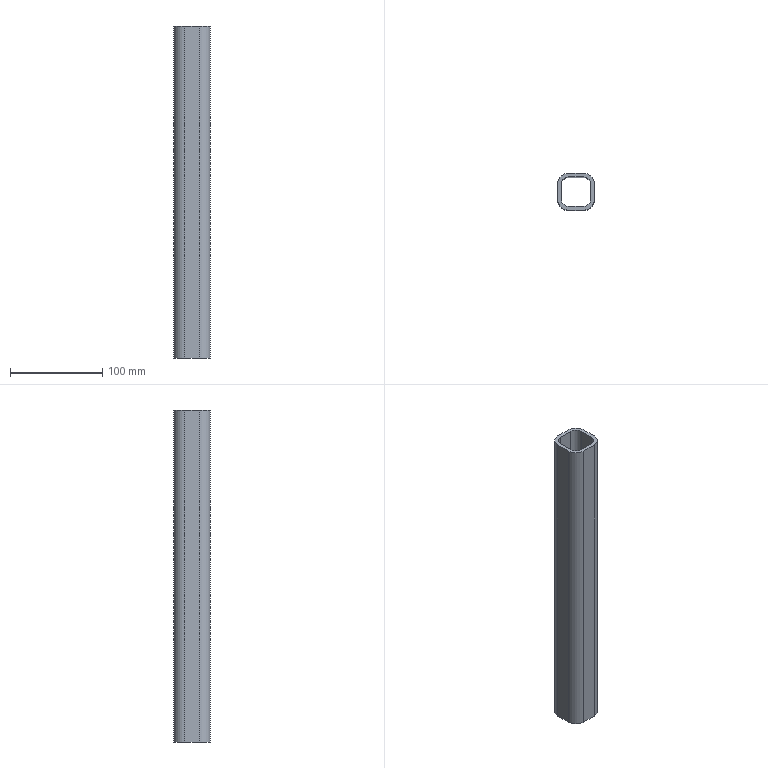Part | SolidWorks | features BaseBody 1 | 1 solid | 18 faces | box 40 x 40 x 360 mm | volume 182638 mm3 | plane 10 | cylinder 8 | commonest cylinder face diameters 16 x4 24 x4
STEP:
#1=CARTESIAN_POINT('',(8.,-20.,0.));
#2=VERTEX_POINT('',#1);
#3=CARTESIAN_POINT('',(20.,-8.,0.));
#4=VERTEX_POINT('',#3);
#5=CARTESIAN_POINT('',(8.,-8.,0.));
#6=DIRECTION('',(0.,0.,1.));
#7=DIRECTION('',(1.,0.,0.));
#8=AXIS2_PLACEMENT_3D('',#5,#6,#7);
#9=CIRCLE('',#8,12.);
#10=EDGE_CURVE('',#2,#4,#9,.T.);
#11=ORIENTED_EDGE('',*,*,#10,.T.);
#12=CARTESIAN_POINT('',(20.,-8.,360.));
#13=VERTEX_POINT('',#12);
#14=CARTESIAN_POINT('',(20.,-8.,0.));
#15=DIRECTION('',(0.,0.,1.));
#16=VECTOR('',#15,1000.);
#17=LINE('',#14,#16);
#18=EDGE_CURVE('',#4,#13,#17,.T.);
#19=ORIENTED_EDGE('',*,*,#18,.T.);
#20=CARTESIAN_POINT('',(8.,-20.,360.));
#21=VERTEX_POINT('',#20);
#22=CARTESIAN_POINT('',(8.,-8.,360.));
#23=DIRECTION('',(0.,0.,-1.));
#24=DIRECTION('',(1.,0.,0.));
#25=AXIS2_PLACEMENT_3D('',#22,#23,#24);
#26=CIRCLE('',#25,12.);
#27=EDGE_CURVE('',#13,#21,#26,.T.);
#28=ORIENTED_EDGE('',*,*,#27,.T.);
#29=CARTESIAN_POINT('',(8.,-20.,0.));
#30=DIRECTION('',(0.,0.,-1.));
#31=VECTOR('',#30,1000.);
#32=LINE('',#29,#31);
#33=EDGE_CURVE('',#21,#2,#32,.T.);
#34=ORIENTED_EDGE('',*,*,#33,.T.);
#35=EDGE_LOOP('',(#11,#19,#28,#34));
#36=FACE_OUTER_BOUND('',#35,.T.);
#37=CARTESIAN_POINT('',(8.,-8.,0.));
#38=DIRECTION('',(0.,0.,1.));
#39=DIRECTION('',(1.,0.,0.));
#40=AXIS2_PLACEMENT_3D('',#37,#38,#39);
#41=CYLINDRICAL_SURFACE('',#40,12.);
#42=ADVANCED_FACE('',(#36),#41,.T.);
#43=CARTESIAN_POINT('',(20.,8.,0.));
#44=VERTEX_POINT('',#43);
#45=CARTESIAN_POINT('',(20.,8.,0.));
#46=DIRECTION('',(0.,1.,0.));
#47=VECTOR('',#46,1000.);
#48=LINE('',#45,#47);
#49=EDGE_CURVE('',#4,#44,#48,.T.);
#50=ORIENTED_EDGE('',*,*,#49,.T.);
#51=CARTESIAN_POINT('',(20.,8.,360.));
#52=VERTEX_POINT('',#51);
#53=CARTESIAN_POINT('',(20.,8.,0.));
#54=DIRECTION('',(0.,0.,1.));
#55=VECTOR('',#54,1000.);
#56=LINE('',#53,#55);
#57=EDGE_CURVE('',#44,#52,#56,.T.);
#58=ORIENTED_EDGE('',*,*,#57,.T.);
#59=CARTESIAN_POINT('',(20.,8.,360.));
#60=DIRECTION('',(0.,-1.,0.));
#61=VECTOR('',#60,1000.);
#62=LINE('',#59,#61);
#63=EDGE_CURVE('',#52,#13,#62,.T.);
#64=ORIENTED_EDGE('',*,*,#63,.T.);
#65=ORIENTED_EDGE('',*,*,#18,.F.);
#66=EDGE_LOOP('',(#50,#58,#64,#65));
#67=FACE_OUTER_BOUND('',#66,.T.);
#68=CARTESIAN_POINT('',(20.,8.,0.));
#69=DIRECTION('',(1.,0.,0.));
#70=DIRECTION('',(0.,1.,0.));
#71=AXIS2_PLACEMENT_3D('',#68,#69,#70);
#72=PLANE('',#71);
#73=ADVANCED_FACE('',(#67),#72,.T.);
#74=CARTESIAN_POINT('',(-16.,8.,0.));
#75=VERTEX_POINT('',#74);
#76=CARTESIAN_POINT('',(-8.,16.,0.));
#77=VERTEX_POINT('',#76);
#78=CARTESIAN_POINT('',(-8.,8.,0.));
#79=DIRECTION('',(0.,0.,-1.));
#80=DIRECTION('',(1.,0.,0.));
#81=AXIS2_PLACEMENT_3D('',#78,#79,#80);
#82=CIRCLE('',#81,8.);
#83=EDGE_CURVE('',#75,#77,#82,.T.);
#84=ORIENTED_EDGE('',*,*,#83,.F.);
#85=CARTESIAN_POINT('',(-16.,-8.,0.));
#86=VERTEX_POINT('',#85);
#87=CARTESIAN_POINT('',(-16.,0.,0.));
#88=DIRECTION('',(0.,1.,0.));
#89=VECTOR('',#88,1000.);
#90=LINE('',#87,#89);
#91=EDGE_CURVE('',#86,#75,#90,.T.);
#92=ORIENTED_EDGE('',*,*,#91,.F.);
#93=CARTESIAN_POINT('',(-8.,-16.,0.));
#94=VERTEX_POINT('',#93);
#95=CARTESIAN_POINT('',(-8.,-8.,0.));
#96=DIRECTION('',(0.,0.,-1.));
#97=DIRECTION('',(1.,0.,0.));
#98=AXIS2_PLACEMENT_3D('',#95,#96,#97);
#99=CIRCLE('',#98,8.);
#100=EDGE_CURVE('',#94,#86,#99,.T.);
#101=ORIENTED_EDGE('',*,*,#100,.F.);
#102=CARTESIAN_POINT('',(8.,-16.,0.));
#103=VERTEX_POINT('',#102);
#104=CARTESIAN_POINT('',(0.,-16.,0.));
#105=DIRECTION('',(-1.,0.,0.));
#106=VECTOR('',#105,1000.);
#107=LINE('',#104,#106);
#108=EDGE_CURVE('',#103,#94,#107,.T.);
#109=ORIENTED_EDGE('',*,*,#108,.F.);
#110=CARTESIAN_POINT('',(16.,-8.,0.));
#111=VERTEX_POINT('',#110);
#112=CARTESIAN_POINT('',(8.,-8.,0.));
#113=DIRECTION('',(0.,0.,-1.));
#114=DIRECTION('',(1.,0.,0.));
#115=AXIS2_PLACEMENT_3D('',#112,#113,#114);
#116=CIRCLE('',#115,8.);
#117=EDGE_CURVE('',#111,#103,#116,.T.);
#118=ORIENTED_EDGE('',*,*,#117,.F.);
#119=CARTESIAN_POINT('',(16.,8.,0.));
#120=VERTEX_POINT('',#119);
#121=CARTESIAN_POINT('',(16.,0.,0.));
#122=DIRECTION('',(0.,-1.,0.));
#123=VECTOR('',#122,1000.);
#124=LINE('',#121,#123);
#125=EDGE_CURVE('',#120,#111,#124,.T.);
#126=ORIENTED_EDGE('',*,*,#125,.F.);
#127=CARTESIAN_POINT('',(8.,16.,0.));
#128=VERTEX_POINT('',#127);
#129=CARTESIAN_POINT('',(8.,8.,0.));
#130=DIRECTION('',(0.,0.,-1.));
#131=DIRECTION('',(1.,0.,0.));
#132=AXIS2_PLACEMENT_3D('',#129,#130,#131);
#133=CIRCLE('',#132,8.);
#134=EDGE_CURVE('',#128,#120,#133,.T.);
#135=ORIENTED_EDGE('',*,*,#134,.F.);
#136=CARTESIAN_POINT('',(0.,16.,0.));
#137=DIRECTION('',(1.,0.,0.));
#138=VECTOR('',#137,1000.);
#139=LINE('',#136,#138);
#140=EDGE_CURVE('',#77,#128,#139,.T.);
#141=ORIENTED_EDGE('',*,*,#140,.F.);
#142=EDGE_LOOP('',(#84,#92,#101,#109,#118,#126,#135,#141));
#143=FACE_BOUND('',#142,.T.);
#144=CARTESIAN_POINT('',(-8.,20.,0.));
#145=VERTEX_POINT('',#144);
#146=CARTESIAN_POINT('',(-20.,8.,0.));
#147=VERTEX_POINT('',#146);
#148=CARTESIAN_POINT('',(-8.,8.,0.));
#149=DIRECTION('',(0.,0.,1.));
#150=DIRECTION('',(1.,0.,0.));
#151=AXIS2_PLACEMENT_3D('',#148,#149,#150);
#152=CIRCLE('',#151,12.);
#153=EDGE_CURVE('',#145,#147,#152,.T.);
#154=ORIENTED_EDGE('',*,*,#153,.F.);
#155=CARTESIAN_POINT('',(8.,20.,0.));
#156=VERTEX_POINT('',#155);
#157=CARTESIAN_POINT('',(0.,20.,0.));
#158=DIRECTION('',(-1.,0.,0.));
#159=VECTOR('',#158,1000.);
#160=LINE('',#157,#159);
#161=EDGE_CURVE('',#156,#145,#160,.T.);
#162=ORIENTED_EDGE('',*,*,#161,.F.);
#163=CARTESIAN_POINT('',(8.,8.,0.));
#164=DIRECTION('',(0.,0.,1.));
#165=DIRECTION('',(1.,0.,0.));
#166=AXIS2_PLACEMENT_3D('',#163,#164,#165);
#167=CIRCLE('',#166,12.);
#168=EDGE_CURVE('',#44,#156,#167,.T.);
#169=ORIENTED_EDGE('',*,*,#168,.F.);
#170=ORIENTED_EDGE('',*,*,#49,.F.);
#171=ORIENTED_EDGE('',*,*,#10,.F.);
#172=CARTESIAN_POINT('',(-8.,-20.,0.));
#173=VERTEX_POINT('',#172);
#174=CARTESIAN_POINT('',(0.,-20.,0.));
#175=DIRECTION('',(1.,0.,0.));
#176=VECTOR('',#175,1000.);
#177=LINE('',#174,#176);
#178=EDGE_CURVE('',#173,#2,#177,.T.);
#179=ORIENTED_EDGE('',*,*,#178,.F.);
#180=CARTESIAN_POINT('',(-20.,-8.,0.));
#181=VERTEX_POINT('',#180);
#182=CARTESIAN_POINT('',(-8.,-8.,0.));
#183=DIRECTION('',(0.,0.,1.));
#184=DIRECTION('',(1.,0.,0.));
#185=AXIS2_PLACEMENT_3D('',#182,#183,#184);
#186=CIRCLE('',#185,12.);
#187=EDGE_CURVE('',#181,#173,#186,.T.);
#188=ORIENTED_EDGE('',*,*,#187,.F.);
#189=CARTESIAN_POINT('',(-20.,0.,0.));
#190=DIRECTION('',(0.,-1.,0.));
#191=VECTOR('',#190,1000.);
#192=LINE('',#189,#191);
#193=EDGE_CURVE('',#147,#181,#192,.T.);
#194=ORIENTED_EDGE('',*,*,#193,.F.);
#195=EDGE_LOOP('',(#154,#162,#169,#170,#171,#179,#188,#194));
#196=FACE_OUTER_BOUND('',#195,.T.);
#197=CARTESIAN_POINT('',(0.,0.,0.));
#198=DIRECTION('',(0.,0.,1.));
#199=DIRECTION('',(1.,0.,0.));
#200=AXIS2_PLACEMENT_3D('',#197,#198,#199);
#201=PLANE('',#200);
#202=ADVANCED_FACE('',(#143,#196),#201,.F.);
#203=ORIENTED_EDGE('',*,*,#178,.T.);
#204=ORIENTED_EDGE('',*,*,#33,.F.);
#205=CARTESIAN_POINT('',(-8.,-20.,360.));
#206=VERTEX_POINT('',#205);
#207=CARTESIAN_POINT('',(8.,-20.,360.));
#208=DIRECTION('',(-1.,0.,0.));
#209=VECTOR('',#208,1000.);
#210=LINE('',#207,#209);
#211=EDGE_CURVE('',#21,#206,#210,.T.);
#212=ORIENTED_EDGE('',*,*,#211,.T.);
#213=CARTESIAN_POINT('',(-8.,-20.,0.));
#214=DIRECTION('',(0.,0.,-1.));
#215=VECTOR('',#214,1000.);
#216=LINE('',#213,#215);
#217=EDGE_CURVE('',#206,#173,#216,.T.);
#218=ORIENTED_EDGE('',*,*,#217,.T.);
#219=EDGE_LOOP('',(#203,#204,#212,#218));
#220=FACE_OUTER_BOUND('',#219,.T.);
#221=CARTESIAN_POINT('',(8.,-20.,0.));
#222=DIRECTION('',(0.,-1.,0.));
#223=DIRECTION('',(1.,0.,0.));
#224=AXIS2_PLACEMENT_3D('',#221,#222,#223);
#225=PLANE('',#224);
#226=ADVANCED_FACE('',(#220),#225,.T.);
#227=CARTESIAN_POINT('',(-16.,-8.,360.));
#228=VERTEX_POINT('',#227);
#229=CARTESIAN_POINT('',(-16.,8.,360.));
#230=VERTEX_POINT('',#229);
#231=CARTESIAN_POINT('',(-16.,0.,360.));
#232=DIRECTION('',(0.,1.,0.));
#233=VECTOR('',#232,1000.);
#234=LINE('',#231,#233);
#235=EDGE_CURVE('',#228,#230,#234,.T.);
#236=ORIENTED_EDGE('',*,*,#235,.T.);
#237=CARTESIAN_POINT('',(-8.,16.,360.));
#238=VERTEX_POINT('',#237);
#239=CARTESIAN_POINT('',(-8.,8.,360.));
#240=DIRECTION('',(0.,0.,-1.));
#241=DIRECTION('',(1.,0.,0.));
#242=AXIS2_PLACEMENT_3D('',#239,#240,#241);
#243=CIRCLE('',#242,8.);
#244=EDGE_CURVE('',#230,#238,#243,.T.);
#245=ORIENTED_EDGE('',*,*,#244,.T.);
#246=CARTESIAN_POINT('',(8.,16.,360.));
#247=VERTEX_POINT('',#246);
#248=CARTESIAN_POINT('',(0.,16.,360.));
#249=DIRECTION('',(1.,0.,0.));
#250=VECTOR('',#249,1000.);
#251=LINE('',#248,#250);
#252=EDGE_CURVE('',#238,#247,#251,.T.);
#253=ORIENTED_EDGE('',*,*,#252,.T.);
#254=CARTESIAN_POINT('',(16.,8.,360.));
#255=VERTEX_POINT('',#254);
#256=CARTESIAN_POINT('',(8.,8.,360.));
#257=DIRECTION('',(0.,0.,-1.));
#258=DIRECTION('',(1.,0.,0.));
#259=AXIS2_PLACEMENT_3D('',#256,#257,#258);
#260=CIRCLE('',#259,8.);
#261=EDGE_CURVE('',#247,#255,#260,.T.);
#262=ORIENTED_EDGE('',*,*,#261,.T.);
#263=CARTESIAN_POINT('',(16.,-8.,360.));
#264=VERTEX_POINT('',#263);
#265=CARTESIAN_POINT('',(16.,0.,360.));
#266=DIRECTION('',(0.,-1.,0.));
#267=VECTOR('',#266,1000.);
#268=LINE('',#265,#267);
#269=EDGE_CURVE('',#255,#264,#268,.T.);
#270=ORIENTED_EDGE('',*,*,#269,.T.);
#271=CARTESIAN_POINT('',(8.,-16.,360.));
#272=VERTEX_POINT('',#271);
#273=CARTESIAN_POINT('',(8.,-8.,360.));
#274=DIRECTION('',(0.,0.,-1.));
#275=DIRECTION('',(1.,0.,0.));
#276=AXIS2_PLACEMENT_3D('',#273,#274,#275);
#277=CIRCLE('',#276,8.);
#278=EDGE_CURVE('',#264,#272,#277,.T.);
#279=ORIENTED_EDGE('',*,*,#278,.T.);
#280=CARTESIAN_POINT('',(-8.,-16.,360.));
#281=VERTEX_POINT('',#280);
#282=CARTESIAN_POINT('',(0.,-16.,360.));
#283=DIRECTION('',(-1.,0.,0.));
#284=VECTOR('',#283,1000.);
#285=LINE('',#282,#284);
#286=EDGE_CURVE('',#272,#281,#285,.T.);
#287=ORIENTED_EDGE('',*,*,#286,.T.);
#288=CARTESIAN_POINT('',(-8.,-8.,360.));
#289=DIRECTION('',(0.,0.,-1.));
#290=DIRECTION('',(1.,0.,0.));
#291=AXIS2_PLACEMENT_3D('',#288,#289,#290);
#292=CIRCLE('',#291,8.);
#293=EDGE_CURVE('',#281,#228,#292,.T.);
#294=ORIENTED_EDGE('',*,*,#293,.T.);
#295=EDGE_LOOP('',(#236,#245,#253,#262,#270,#279,#287,#294));
#296=FACE_BOUND('',#295,.T.);
#297=CARTESIAN_POINT('',(8.,20.,360.));
#298=VERTEX_POINT('',#297);
#299=CARTESIAN_POINT('',(-8.,20.,360.));
#300=VERTEX_POINT('',#299);
#301=CARTESIAN_POINT('',(0.,20.,360.));
#302=DIRECTION('',(-1.,0.,0.));
#303=VECTOR('',#302,1000.);
#304=LINE('',#301,#303);
#305=EDGE_CURVE('',#298,#300,#304,.T.);
#306=ORIENTED_EDGE('',*,*,#305,.T.);
#307=CARTESIAN_POINT('',(-20.,8.,360.));
#308=VERTEX_POINT('',#307);
#309=CARTESIAN_POINT('',(-8.,8.,360.));
#310=DIRECTION('',(0.,0.,1.));
#311=DIRECTION('',(1.,0.,0.));
#312=AXIS2_PLACEMENT_3D('',#309,#310,#311);
#313=CIRCLE('',#312,12.);
#314=EDGE_CURVE('',#300,#308,#313,.T.);
#315=ORIENTED_EDGE('',*,*,#314,.T.);
#316=CARTESIAN_POINT('',(-20.,-8.,360.));
#317=VERTEX_POINT('',#316);
#318=CARTESIAN_POINT('',(-20.,0.,360.));
#319=DIRECTION('',(0.,-1.,0.));
#320=VECTOR('',#319,1000.);
#321=LINE('',#318,#320);
#322=EDGE_CURVE('',#308,#317,#321,.T.);
#323=ORIENTED_EDGE('',*,*,#322,.T.);
#324=CARTESIAN_POINT('',(-8.,-8.,360.));
#325=DIRECTION('',(0.,0.,1.));
#326=DIRECTION('',(1.,0.,0.));
#327=AXIS2_PLACEMENT_3D('',#324,#325,#326);
#328=CIRCLE('',#327,12.);
#329=EDGE_CURVE('',#317,#206,#328,.T.);
#330=ORIENTED_EDGE('',*,*,#329,.T.);
#331=ORIENTED_EDGE('',*,*,#211,.F.);
#332=ORIENTED_EDGE('',*,*,#27,.F.);
#333=ORIENTED_EDGE('',*,*,#63,.F.);
#334=CARTESIAN_POINT('',(8.,8.,360.));
#335=DIRECTION('',(0.,0.,1.));
#336=DIRECTION('',(1.,0.,0.));
#337=AXIS2_PLACEMENT_3D('',#334,#335,#336);
#338=CIRCLE('',#337,12.);
#339=EDGE_CURVE('',#52,#298,#338,.T.);
#340=ORIENTED_EDGE('',*,*,#339,.T.);
#341=EDGE_LOOP('',(#306,#315,#323,#330,#331,#332,#333,#340));
#342=FACE_OUTER_BOUND('',#341,.T.);
#343=CARTESIAN_POINT('',(0.,0.,360.));
#344=DIRECTION('',(0.,0.,1.));
#345=DIRECTION('',(1.,0.,0.));
#346=AXIS2_PLACEMENT_3D('',#343,#344,#345);
#347=PLANE('',#346);
#348=ADVANCED_FACE('',(#296,#342),#347,.T.);
#349=ORIENTED_EDGE('',*,*,#168,.T.);
#350=CARTESIAN_POINT('',(8.,20.,0.));
#351=DIRECTION('',(0.,0.,1.));
#352=VECTOR('',#351,1000.);
#353=LINE('',#350,#352);
#354=EDGE_CURVE('',#156,#298,#353,.T.);
#355=ORIENTED_EDGE('',*,*,#354,.T.);
#356=ORIENTED_EDGE('',*,*,#339,.F.);
#357=ORIENTED_EDGE('',*,*,#57,.F.);
#358=EDGE_LOOP('',(#349,#355,#356,#357));
#359=FACE_OUTER_BOUND('',#358,.T.);
#360=CARTESIAN_POINT('',(8.,8.,0.));
#361=DIRECTION('',(0.,0.,1.));
#362=DIRECTION('',(1.,0.,0.));
#363=AXIS2_PLACEMENT_3D('',#360,#361,#362);
#364=CYLINDRICAL_SURFACE('',#363,12.);
#365=ADVANCED_FACE('',(#359),#364,.T.);
#366=CARTESIAN_POINT('',(-8.,16.,0.));
#367=DIRECTION('',(0.,0.,1.));
#368=VECTOR('',#367,1000.);
#369=LINE('',#366,#368);
#370=EDGE_CURVE('',#77,#238,#369,.T.);
#371=ORIENTED_EDGE('',*,*,#370,.F.);
#372=ORIENTED_EDGE('',*,*,#140,.T.);
#373=CARTESIAN_POINT('',(8.,16.,0.));
#374=DIRECTION('',(0.,0.,-1.));
#375=VECTOR('',#374,1000.);
#376=LINE('',#373,#375);
#377=EDGE_CURVE('',#247,#128,#376,.T.);
#378=ORIENTED_EDGE('',*,*,#377,.F.);
#379=ORIENTED_EDGE('',*,*,#252,.F.);
#380=EDGE_LOOP('',(#371,#372,#378,#379));
#381=FACE_OUTER_BOUND('',#380,.T.);
#382=CARTESIAN_POINT('',(-8.,16.,0.));
#383=DIRECTION('',(0.,1.,0.));
#384=DIRECTION('',(-1.,0.,0.));
#385=AXIS2_PLACEMENT_3D('',#382,#383,#384);
#386=PLANE('',#385);
#387=ADVANCED_FACE('',(#381),#386,.F.);
#388=CARTESIAN_POINT('',(-16.,8.,0.));
#389=DIRECTION('',(0.,0.,1.));
#390=VECTOR('',#389,1000.);
#391=LINE('',#388,#390);
#392=EDGE_CURVE('',#75,#230,#391,.T.);
#393=ORIENTED_EDGE('',*,*,#392,.F.);
#394=ORIENTED_EDGE('',*,*,#83,.T.);
#395=ORIENTED_EDGE('',*,*,#370,.T.);
#396=ORIENTED_EDGE('',*,*,#244,.F.);
#397=EDGE_LOOP('',(#393,#394,#395,#396));
#398=FACE_OUTER_BOUND('',#397,.T.);
#399=CARTESIAN_POINT('',(-8.,8.,0.));
#400=DIRECTION('',(0.,0.,1.));
#401=DIRECTION('',(1.,0.,0.));
#402=AXIS2_PLACEMENT_3D('',#399,#400,#401);
#403=CYLINDRICAL_SURFACE('',#402,8.);
#404=ADVANCED_FACE('',(#398),#403,.F.);
#405=CARTESIAN_POINT('',(-16.,-8.,0.));
#406=DIRECTION('',(0.,0.,1.));
#407=VECTOR('',#406,1000.);
#408=LINE('',#405,#407);
#409=EDGE_CURVE('',#86,#228,#408,.T.);
#410=ORIENTED_EDGE('',*,*,#409,.F.);
#411=ORIENTED_EDGE('',*,*,#91,.T.);
#412=ORIENTED_EDGE('',*,*,#392,.T.);
#413=ORIENTED_EDGE('',*,*,#235,.F.);
#414=EDGE_LOOP('',(#410,#411,#412,#413));
#415=FACE_OUTER_BOUND('',#414,.T.);
#416=CARTESIAN_POINT('',(-16.,-8.,0.));
#417=DIRECTION('',(-1.,0.,0.));
#418=DIRECTION('',(0.,-1.,0.));
#419=AXIS2_PLACEMENT_3D('',#416,#417,#418);
#420=PLANE('',#419);
#421=ADVANCED_FACE('',(#415),#420,.F.);
#422=CARTESIAN_POINT('',(-8.,-16.,0.));
#423=DIRECTION('',(0.,0.,1.));
#424=VECTOR('',#423,1000.);
#425=LINE('',#422,#424);
#426=EDGE_CURVE('',#94,#281,#425,.T.);
#427=ORIENTED_EDGE('',*,*,#426,.F.);
#428=ORIENTED_EDGE('',*,*,#100,.T.);
#429=ORIENTED_EDGE('',*,*,#409,.T.);
#430=ORIENTED_EDGE('',*,*,#293,.F.);
#431=EDGE_LOOP('',(#427,#428,#429,#430));
#432=FACE_OUTER_BOUND('',#431,.T.);
#433=CARTESIAN_POINT('',(-8.,-8.,0.));
#434=DIRECTION('',(0.,0.,1.));
#435=DIRECTION('',(1.,0.,0.));
#436=AXIS2_PLACEMENT_3D('',#433,#434,#435);
#437=CYLINDRICAL_SURFACE('',#436,8.);
#438=ADVANCED_FACE('',(#432),#437,.F.);
#439=CARTESIAN_POINT('',(8.,-16.,0.));
#440=DIRECTION('',(0.,0.,1.));
#441=VECTOR('',#440,1000.);
#442=LINE('',#439,#441);
#443=EDGE_CURVE('',#103,#272,#442,.T.);
#444=ORIENTED_EDGE('',*,*,#443,.F.);
#445=ORIENTED_EDGE('',*,*,#108,.T.);
#446=ORIENTED_EDGE('',*,*,#426,.T.);
#447=ORIENTED_EDGE('',*,*,#286,.F.);
#448=EDGE_LOOP('',(#444,#445,#446,#447));
#449=FACE_OUTER_BOUND('',#448,.T.);
#450=CARTESIAN_POINT('',(8.,-16.,0.));
#451=DIRECTION('',(0.,-1.,0.));
#452=DIRECTION('',(1.,0.,0.));
#453=AXIS2_PLACEMENT_3D('',#450,#451,#452);
#454=PLANE('',#453);
#455=ADVANCED_FACE('',(#449),#454,.F.);
#456=CARTESIAN_POINT('',(16.,-8.,0.));
#457=DIRECTION('',(0.,0.,1.));
#458=VECTOR('',#457,1000.);
#459=LINE('',#456,#458);
#460=EDGE_CURVE('',#111,#264,#459,.T.);
#461=ORIENTED_EDGE('',*,*,#460,.F.);
#462=ORIENTED_EDGE('',*,*,#117,.T.);
#463=ORIENTED_EDGE('',*,*,#443,.T.);
#464=ORIENTED_EDGE('',*,*,#278,.F.);
#465=EDGE_LOOP('',(#461,#462,#463,#464));
#466=FACE_OUTER_BOUND('',#465,.T.);
#467=CARTESIAN_POINT('',(8.,-8.,0.));
#468=DIRECTION('',(0.,0.,1.));
#469=DIRECTION('',(1.,0.,0.));
#470=AXIS2_PLACEMENT_3D('',#467,#468,#469);
#471=CYLINDRICAL_SURFACE('',#470,8.);
#472=ADVANCED_FACE('',(#466),#471,.F.);
#473=CARTESIAN_POINT('',(16.,8.,0.));
#474=DIRECTION('',(0.,0.,1.));
#475=VECTOR('',#474,1000.);
#476=LINE('',#473,#475);
#477=EDGE_CURVE('',#120,#255,#476,.T.);
#478=ORIENTED_EDGE('',*,*,#477,.F.);
#479=ORIENTED_EDGE('',*,*,#125,.T.);
#480=ORIENTED_EDGE('',*,*,#460,.T.);
#481=ORIENTED_EDGE('',*,*,#269,.F.);
#482=EDGE_LOOP('',(#478,#479,#480,#481));
#483=FACE_OUTER_BOUND('',#482,.T.);
#484=CARTESIAN_POINT('',(16.,8.,0.));
#485=DIRECTION('',(1.,0.,0.));
#486=DIRECTION('',(0.,0.,-1.));
#487=AXIS2_PLACEMENT_3D('',#484,#485,#486);
#488=PLANE('',#487);
#489=ADVANCED_FACE('',(#483),#488,.F.);
#490=ORIENTED_EDGE('',*,*,#377,.T.);
#491=ORIENTED_EDGE('',*,*,#134,.T.);
#492=ORIENTED_EDGE('',*,*,#477,.T.);
#493=ORIENTED_EDGE('',*,*,#261,.F.);
#494=EDGE_LOOP('',(#490,#491,#492,#493));
#495=FACE_OUTER_BOUND('',#494,.T.);
#496=CARTESIAN_POINT('',(8.,8.,0.));
#497=DIRECTION('',(0.,0.,1.));
#498=DIRECTION('',(1.,0.,0.));
#499=AXIS2_PLACEMENT_3D('',#496,#497,#498);
#500=CYLINDRICAL_SURFACE('',#499,8.);
#501=ADVANCED_FACE('',(#495),#500,.F.);
#502=ORIENTED_EDGE('',*,*,#193,.T.);
#503=CARTESIAN_POINT('',(-20.,-8.,0.));
#504=DIRECTION('',(0.,0.,1.));
#505=VECTOR('',#504,1000.);
#506=LINE('',#503,#505);
#507=EDGE_CURVE('',#181,#317,#506,.T.);
#508=ORIENTED_EDGE('',*,*,#507,.T.);
#509=ORIENTED_EDGE('',*,*,#322,.F.);
#510=CARTESIAN_POINT('',(-20.,8.,0.));
#511=DIRECTION('',(0.,0.,-1.));
#512=VECTOR('',#511,1000.);
#513=LINE('',#510,#512);
#514=EDGE_CURVE('',#308,#147,#513,.T.);
#515=ORIENTED_EDGE('',*,*,#514,.T.);
#516=EDGE_LOOP('',(#502,#508,#509,#515));
#517=FACE_OUTER_BOUND('',#516,.T.);
#518=CARTESIAN_POINT('',(-20.,-8.,0.));
#519=DIRECTION('',(-1.,0.,0.));
#520=DIRECTION('',(0.,-1.,0.));
#521=AXIS2_PLACEMENT_3D('',#518,#519,#520);
#522=PLANE('',#521);
#523=ADVANCED_FACE('',(#517),#522,.T.);
#524=ORIENTED_EDGE('',*,*,#153,.T.);
#525=ORIENTED_EDGE('',*,*,#514,.F.);
#526=ORIENTED_EDGE('',*,*,#314,.F.);
#527=CARTESIAN_POINT('',(-8.,20.,0.));
#528=DIRECTION('',(0.,0.,-1.));
#529=VECTOR('',#528,1000.);
#530=LINE('',#527,#529);
#531=EDGE_CURVE('',#300,#145,#530,.T.);
#532=ORIENTED_EDGE('',*,*,#531,.T.);
#533=EDGE_LOOP('',(#524,#525,#526,#532));
#534=FACE_OUTER_BOUND('',#533,.T.);
#535=CARTESIAN_POINT('',(-8.,8.,0.));
#536=DIRECTION('',(0.,0.,1.));
#537=DIRECTION('',(1.,0.,0.));
#538=AXIS2_PLACEMENT_3D('',#535,#536,#537);
#539=CYLINDRICAL_SURFACE('',#538,12.);
#540=ADVANCED_FACE('',(#534),#539,.T.);
#541=ORIENTED_EDGE('',*,*,#161,.T.);
#542=ORIENTED_EDGE('',*,*,#531,.F.);
#543=ORIENTED_EDGE('',*,*,#305,.F.);
#544=ORIENTED_EDGE('',*,*,#354,.F.);
#545=EDGE_LOOP('',(#541,#542,#543,#544));
#546=FACE_OUTER_BOUND('',#545,.T.);
#547=CARTESIAN_POINT('',(-8.,20.,0.));
#548=DIRECTION('',(0.,1.,0.));
#549=DIRECTION('',(0.,0.,1.));
#550=AXIS2_PLACEMENT_3D('',#547,#548,#549);
#551=PLANE('',#550);
#552=ADVANCED_FACE('',(#546),#551,.T.);
#553=ORIENTED_EDGE('',*,*,#187,.T.);
#554=ORIENTED_EDGE('',*,*,#217,.F.);
#555=ORIENTED_EDGE('',*,*,#329,.F.);
#556=ORIENTED_EDGE('',*,*,#507,.F.);
#557=EDGE_LOOP('',(#553,#554,#555,#556));
#558=FACE_OUTER_BOUND('',#557,.T.);
#559=CARTESIAN_POINT('',(-8.,-8.,0.));
#560=DIRECTION('',(0.,0.,1.));
#561=DIRECTION('',(1.,0.,0.));
#562=AXIS2_PLACEMENT_3D('',#559,#560,#561);
#563=CYLINDRICAL_SURFACE('',#562,12.);
#564=ADVANCED_FACE('',(#558),#563,.T.);
#565=CLOSED_SHELL('',(#42,#73,#202,#226,#348,#365,#387,#404,#421,#438,#455,#472,#489,#501,#523,#540,#552,#564));
#566=MANIFOLD_SOLID_BREP('',#565);
#567=CARTESIAN_POINT('',(0.,0.,0.));
#568=DIRECTION('',(0.,0.,1.));
#569=DIRECTION('',(1.,0.,0.));
#570=AXIS2_PLACEMENT_3D('',#567,#568,#569);
#571=(LENGTH_UNIT()NAMED_UNIT(*)SI_UNIT(.MILLI.,.METRE.));
#572=UNCERTAINTY_MEASURE_WITH_UNIT(LENGTH_MEASURE(0.00001),#571,'','');
#573=(NAMED_UNIT(*)PLANE_ANGLE_UNIT()SI_UNIT($,.RADIAN.));
#574=(NAMED_UNIT(*)SI_UNIT($,.STERADIAN.)SOLID_ANGLE_UNIT());
#575=(GEOMETRIC_REPRESENTATION_CONTEXT(3)GLOBAL_UNCERTAINTY_ASSIGNED_CONTEXT((#572))GLOBAL_UNIT_ASSIGNED_CONTEXT((#571,#573,#574))REPRESENTATION_CONTEXT('',''));
#576=ADVANCED_BREP_SHAPE_REPRESENTATION('',(#566,#570),#575);